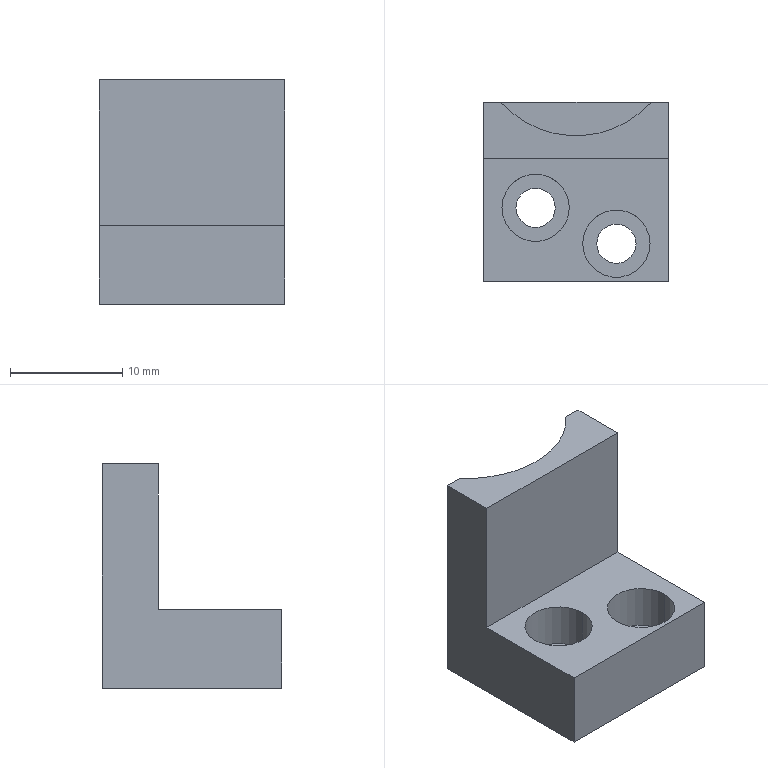Part | SolidWorks | features ICE 3, Extrusion 1, HoleWzd 1 | 1 solid | 93 faces | box 16.5 x 16 x 20 mm | volume 2274 mm3 | plane 56 | spline 28 | cylinder 9 | commonest cylinder face diameters 3.5 x4 6 x4 18 x1